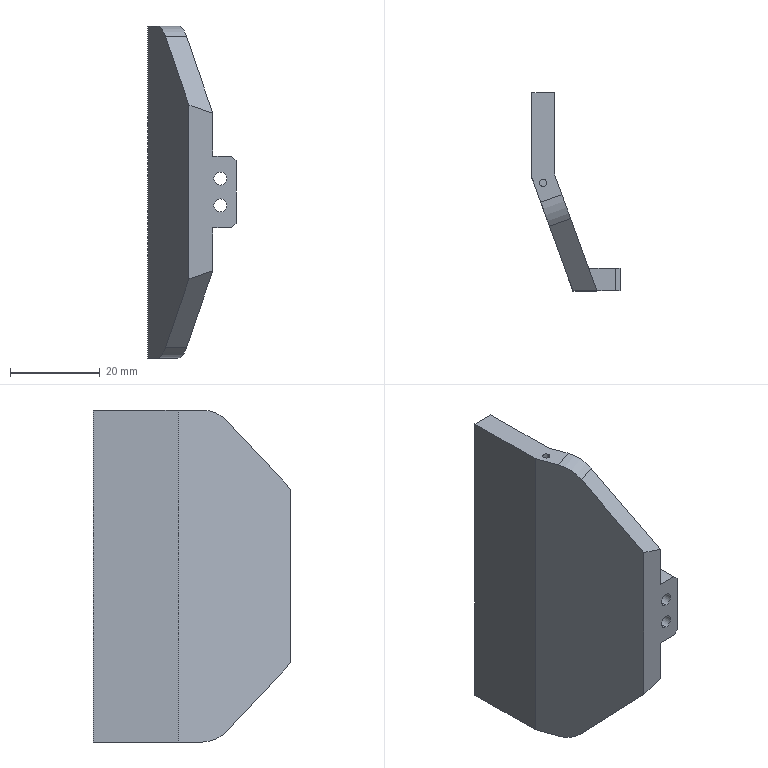NC program | NX | posted with a generic post | part box 19.643 x 44.061 x 74 mm
Whole program:
N10 G17 G21 G94 G90
(SPOT_FACING_1 , TOOL : D4点钻)
N12 T05 M6
N14 G54
N16 G17 G0 G90 X0. Y13. B0. C0. S3000 M3
N18 G43 Z30. H5
N20 G94 G82 G99 Z-1. F200. P200 R6.
N22 G80
N24 G0 X0. Y13. Z30.
N26 M5
(SPOT_FACING_1_COPY , TOOL : D1.8钻头)
N28 T09 M6
N30 G54
N32 G17 G0 G90 X0. Y13. B0. C0. S3000 M3
N34 G43 Z30. H9
N36 G94 G83 G99 Z-8. F150. Q1. R6.
N38 G80
N40 G0 X0. Y13. Z30.
N42 M5
N44 M2